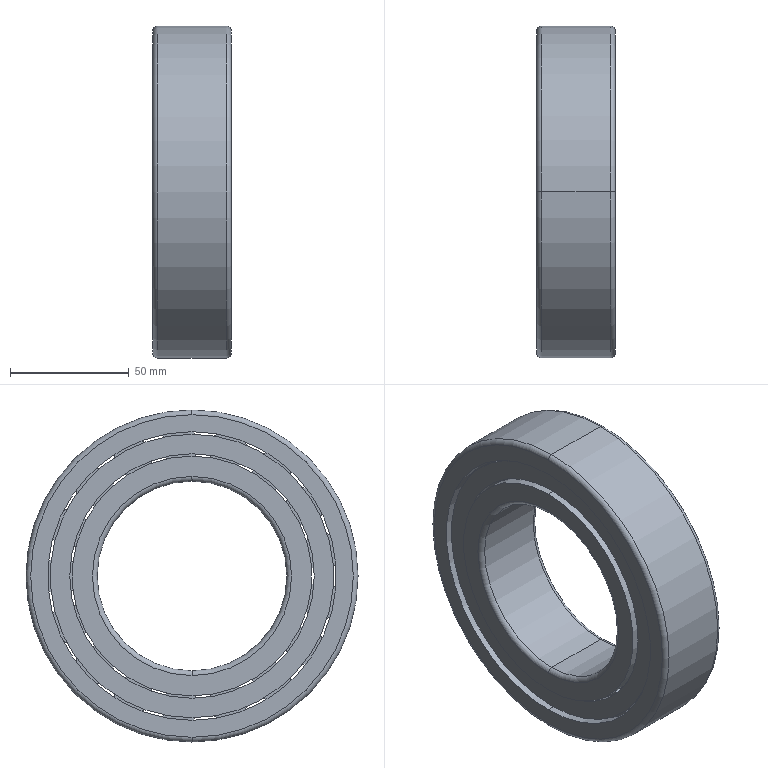Part | SolidWorks | features MBimport 1 | 21 solids | 115 faces | box 33 x 140 x 140 mm | volume 264918 mm3 | cylinder 60 | plane 47 | torus 8 | commonest cylinder face diameters 16 x34 103.06 x4 119.54 x4 121.7 x4 80 x2 95.3 x2